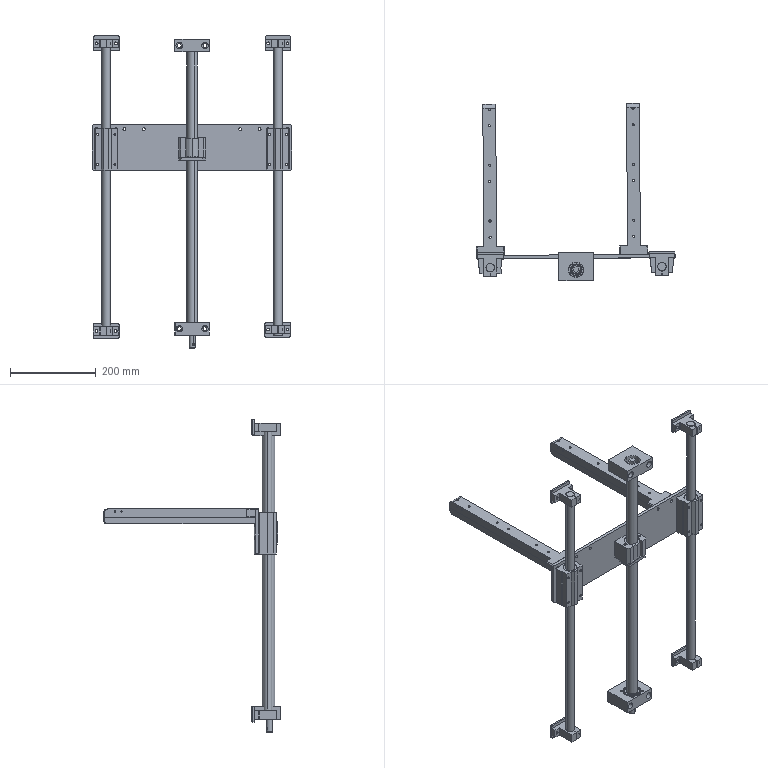Part | SolidWorks | 24 solids | 942 faces | box 465.166 x 413.18 x 727.5 mm | volume 2675424 mm3 | cylinder 391 | plane 287 | cone 150 | spline 114 | commonest cylinder face diameters 5 x48 6.6 x44 20 x34 4.2 x32 1 x24 6.8 x24